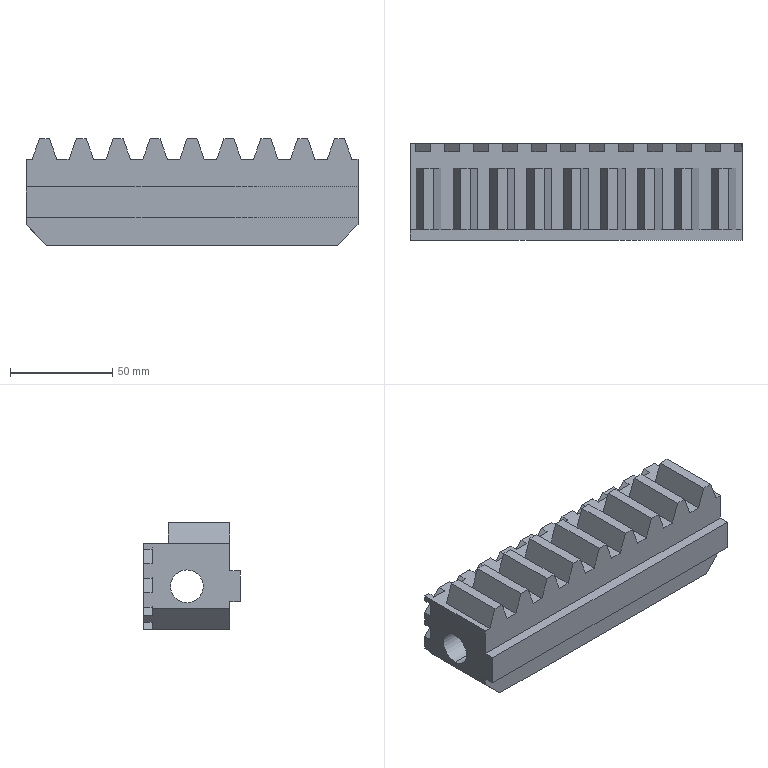Part | SolidWorks | features ICE 4, Chamfer 1, Extrusion 1 | 1 solid | 106 faces | box 162 x 47 x 52 mm | volume 270321 mm3 | plane 104 | cylinder 2 | commonest cylinder face diameters 16 x2